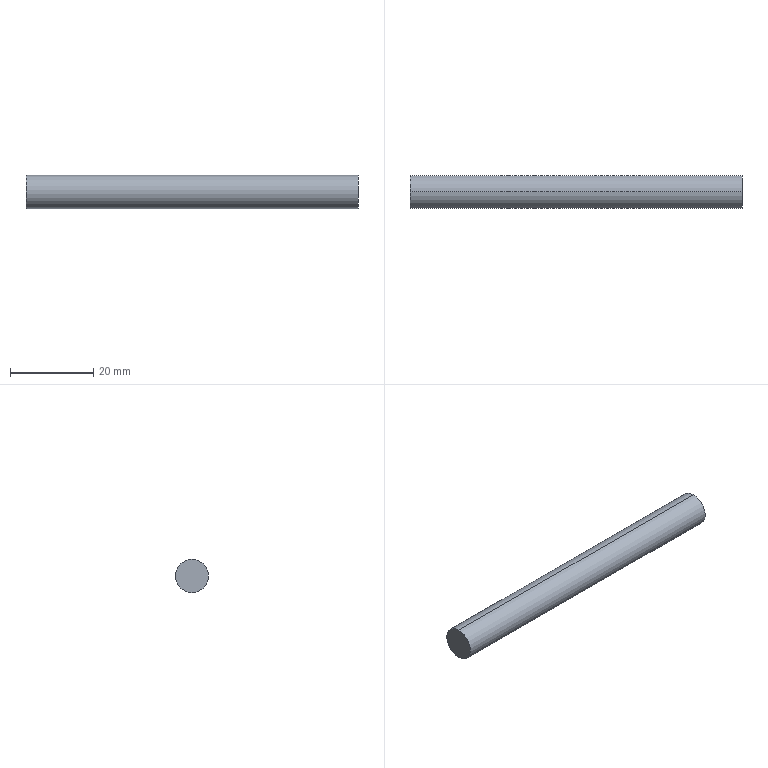Part | SolidWorks | features 3DProfileFeature 1, HoleWzd 1, Revolution 1 | 1 solid | 9 faces | box 79.975 x 8 x 8 mm | volume 3311 mm3 | cylinder 4 | cone 4 | plane 1 | commonest cylinder face diameters 6.8 x2 8 x2
STEP:
#1=CARTESIAN_POINT('',(61.25,0.,3.4));
#2=VERTEX_POINT('',#1);
#3=CARTESIAN_POINT('',(61.25,0.,-3.4));
#4=VERTEX_POINT('',#3);
#5=CARTESIAN_POINT('',(61.25,0.,0.));
#6=DIRECTION('',(1.,0.,0.));
#7=DIRECTION('',(0.,0.,-1.));
#8=AXIS2_PLACEMENT_3D('',#5,#6,#7);
#9=CIRCLE('',#8,3.4);
#10=EDGE_CURVE('',#2,#4,#9,.T.);
#11=ORIENTED_EDGE('',*,*,#10,.F.);
#12=CARTESIAN_POINT('',(79.375,0.,3.4));
#13=VERTEX_POINT('',#12);
#14=CARTESIAN_POINT('',(80.,0.,3.4));
#15=DIRECTION('',(1.,0.,0.));
#16=VECTOR('',#15,1000.);
#17=LINE('',#14,#16);
#18=EDGE_CURVE('',#2,#13,#17,.T.);
#19=ORIENTED_EDGE('',*,*,#18,.T.);
#20=CARTESIAN_POINT('',(79.375,0.,-3.4));
#21=VERTEX_POINT('',#20);
#22=CARTESIAN_POINT('',(79.375,0.,0.));
#23=DIRECTION('',(1.,0.,0.));
#24=DIRECTION('',(0.,0.,-1.));
#25=AXIS2_PLACEMENT_3D('',#22,#23,#24);
#26=CIRCLE('',#25,3.4);
#27=EDGE_CURVE('',#13,#21,#26,.T.);
#28=ORIENTED_EDGE('',*,*,#27,.T.);
#29=CARTESIAN_POINT('',(80.,0.,-3.4));
#30=DIRECTION('',(1.,0.,0.));
#31=VECTOR('',#30,1000.);
#32=LINE('',#29,#31);
#33=EDGE_CURVE('',#4,#21,#32,.T.);
#34=ORIENTED_EDGE('',*,*,#33,.F.);
#35=EDGE_LOOP('',(#11,#19,#28,#34));
#36=FACE_OUTER_BOUND('',#35,.T.);
#37=CARTESIAN_POINT('',(80.,0.,0.));
#38=DIRECTION('',(1.,0.,0.));
#39=DIRECTION('',(0.,0.,-1.));
#40=AXIS2_PLACEMENT_3D('',#37,#38,#39);
#41=CYLINDRICAL_SURFACE('',#40,3.4);
#42=ADVANCED_FACE('',(#36),#41,.F.);
#43=CARTESIAN_POINT('',(59.207,0.,0.));
#44=VERTEX_POINT('',#43);
#45=CARTESIAN_POINT('',(61.25,0.,-3.4));
#46=DIRECTION('',(0.515,0.,-0.8572));
#47=VECTOR('',#46,1000.);
#48=LINE('',#45,#47);
#49=EDGE_CURVE('',#44,#4,#48,.T.);
#50=ORIENTED_EDGE('',*,*,#49,.F.);
#51=CARTESIAN_POINT('',(61.25,0.,3.4));
#52=DIRECTION('',(0.515,0.,0.8572));
#53=VECTOR('',#52,1000.);
#54=LINE('',#51,#53);
#55=EDGE_CURVE('',#44,#2,#54,.T.);
#56=ORIENTED_EDGE('',*,*,#55,.T.);
#57=ORIENTED_EDGE('',*,*,#10,.T.);
#58=EDGE_LOOP('',(#50,#56,#57));
#59=FACE_OUTER_BOUND('',#58,.T.);
#60=CARTESIAN_POINT('',(61.25,0.,0.));
#61=DIRECTION('',(1.,0.,0.));
#62=DIRECTION('',(0.,0.,-1.));
#63=AXIS2_PLACEMENT_3D('',#60,#61,#62);
#64=CONICAL_SURFACE('',#63,3.4,1.03);
#65=ADVANCED_FACE('',(#59),#64,.F.);
#66=ORIENTED_EDGE('',*,*,#27,.F.);
#67=CARTESIAN_POINT('',(79.975,0.,4.));
#68=VERTEX_POINT('',#67);
#69=CARTESIAN_POINT('',(80.,0.,4.025));
#70=DIRECTION('',(0.7071,0.,0.7071));
#71=VECTOR('',#70,1000.);
#72=LINE('',#69,#71);
#73=EDGE_CURVE('',#13,#68,#72,.T.);
#74=ORIENTED_EDGE('',*,*,#73,.T.);
#75=CARTESIAN_POINT('',(79.975,0.,-4.));
#76=VERTEX_POINT('',#75);
#77=CARTESIAN_POINT('',(79.975,0.,0.));
#78=DIRECTION('',(-1.,0.,0.));
#79=DIRECTION('',(0.,0.,-1.));
#80=AXIS2_PLACEMENT_3D('',#77,#78,#79);
#81=CIRCLE('',#80,4.);
#82=EDGE_CURVE('',#76,#68,#81,.T.);
#83=ORIENTED_EDGE('',*,*,#82,.F.);
#84=CARTESIAN_POINT('',(80.,0.,-4.025));
#85=DIRECTION('',(0.7071,0.,-0.7071));
#86=VECTOR('',#85,1000.);
#87=LINE('',#84,#86);
#88=EDGE_CURVE('',#21,#76,#87,.T.);
#89=ORIENTED_EDGE('',*,*,#88,.F.);
#90=EDGE_LOOP('',(#66,#74,#83,#89));
#91=FACE_OUTER_BOUND('',#90,.T.);
#92=CARTESIAN_POINT('',(80.,0.,0.));
#93=DIRECTION('',(1.,0.,0.));
#94=DIRECTION('',(0.,0.,-1.));
#95=AXIS2_PLACEMENT_3D('',#92,#93,#94);
#96=CONICAL_SURFACE('',#95,4.025,0.7854);
#97=ADVANCED_FACE('',(#91),#96,.F.);
#98=CARTESIAN_POINT('',(79.975,0.,0.));
#99=DIRECTION('',(-1.,0.,0.));
#100=DIRECTION('',(0.,0.,-1.));
#101=AXIS2_PLACEMENT_3D('',#98,#99,#100);
#102=CIRCLE('',#101,4.);
#103=EDGE_CURVE('',#68,#76,#102,.T.);
#104=ORIENTED_EDGE('',*,*,#103,.T.);
#105=CARTESIAN_POINT('',(0.,0.,-4.));
#106=VERTEX_POINT('',#105);
#107=CARTESIAN_POINT('',(0.,0.,-4.));
#108=DIRECTION('',(-1.,0.,0.));
#109=VECTOR('',#108,1000.);
#110=LINE('',#107,#109);
#111=EDGE_CURVE('',#76,#106,#110,.T.);
#112=ORIENTED_EDGE('',*,*,#111,.T.);
#113=CARTESIAN_POINT('',(0.,0.,4.));
#114=VERTEX_POINT('',#113);
#115=CARTESIAN_POINT('',(0.,0.,0.));
#116=DIRECTION('',(-1.,0.,0.));
#117=DIRECTION('',(0.,0.,1.));
#118=AXIS2_PLACEMENT_3D('',#115,#116,#117);
#119=CIRCLE('',#118,4.);
#120=EDGE_CURVE('',#114,#106,#119,.T.);
#121=ORIENTED_EDGE('',*,*,#120,.F.);
#122=CARTESIAN_POINT('',(0.,0.,4.));
#123=DIRECTION('',(-1.,0.,0.));
#124=VECTOR('',#123,1000.);
#125=LINE('',#122,#124);
#126=EDGE_CURVE('',#68,#114,#125,.T.);
#127=ORIENTED_EDGE('',*,*,#126,.F.);
#128=EDGE_LOOP('',(#104,#112,#121,#127));
#129=FACE_OUTER_BOUND('',#128,.T.);
#130=CARTESIAN_POINT('',(0.,0.,0.));
#131=DIRECTION('',(-1.,0.,0.));
#132=DIRECTION('',(0.,0.,1.));
#133=AXIS2_PLACEMENT_3D('',#130,#131,#132);
#134=CYLINDRICAL_SURFACE('',#133,4.);
#135=ADVANCED_FACE('',(#129),#134,.T.);
#136=ORIENTED_EDGE('',*,*,#120,.T.);
#137=CARTESIAN_POINT('',(0.,0.,0.));
#138=DIRECTION('',(-1.,0.,0.));
#139=DIRECTION('',(0.,0.,1.));
#140=AXIS2_PLACEMENT_3D('',#137,#138,#139);
#141=CIRCLE('',#140,4.);
#142=EDGE_CURVE('',#106,#114,#141,.T.);
#143=ORIENTED_EDGE('',*,*,#142,.T.);
#144=EDGE_LOOP('',(#136,#143));
#145=FACE_OUTER_BOUND('',#144,.T.);
#146=CARTESIAN_POINT('',(0.,0.,0.));
#147=DIRECTION('',(1.,0.,0.));
#148=DIRECTION('',(0.,0.,-1.));
#149=AXIS2_PLACEMENT_3D('',#146,#147,#148);
#150=PLANE('',#149);
#151=ADVANCED_FACE('',(#145),#150,.F.);
#152=ORIENTED_EDGE('',*,*,#111,.F.);
#153=ORIENTED_EDGE('',*,*,#82,.T.);
#154=ORIENTED_EDGE('',*,*,#126,.T.);
#155=ORIENTED_EDGE('',*,*,#142,.F.);
#156=EDGE_LOOP('',(#152,#153,#154,#155));
#157=FACE_OUTER_BOUND('',#156,.T.);
#158=CARTESIAN_POINT('',(0.,0.,0.));
#159=DIRECTION('',(-1.,0.,0.));
#160=DIRECTION('',(0.,0.,1.));
#161=AXIS2_PLACEMENT_3D('',#158,#159,#160);
#162=CYLINDRICAL_SURFACE('',#161,4.);
#163=ADVANCED_FACE('',(#157),#162,.T.);
#164=ORIENTED_EDGE('',*,*,#73,.F.);
#165=CARTESIAN_POINT('',(79.375,0.,0.));
#166=DIRECTION('',(1.,0.,0.));
#167=DIRECTION('',(0.,0.,-1.));
#168=AXIS2_PLACEMENT_3D('',#165,#166,#167);
#169=CIRCLE('',#168,3.4);
#170=EDGE_CURVE('',#21,#13,#169,.T.);
#171=ORIENTED_EDGE('',*,*,#170,.F.);
#172=ORIENTED_EDGE('',*,*,#88,.T.);
#173=ORIENTED_EDGE('',*,*,#103,.F.);
#174=EDGE_LOOP('',(#164,#171,#172,#173));
#175=FACE_OUTER_BOUND('',#174,.T.);
#176=CARTESIAN_POINT('',(80.,0.,0.));
#177=DIRECTION('',(1.,0.,0.));
#178=DIRECTION('',(0.,0.,-1.));
#179=AXIS2_PLACEMENT_3D('',#176,#177,#178);
#180=CONICAL_SURFACE('',#179,4.025,0.7854);
#181=ADVANCED_FACE('',(#175),#180,.F.);
#182=ORIENTED_EDGE('',*,*,#55,.F.);
#183=ORIENTED_EDGE('',*,*,#49,.T.);
#184=CARTESIAN_POINT('',(61.25,0.,0.));
#185=DIRECTION('',(1.,0.,0.));
#186=DIRECTION('',(0.,0.,-1.));
#187=AXIS2_PLACEMENT_3D('',#184,#185,#186);
#188=CIRCLE('',#187,3.4);
#189=EDGE_CURVE('',#4,#2,#188,.T.);
#190=ORIENTED_EDGE('',*,*,#189,.T.);
#191=EDGE_LOOP('',(#182,#183,#190));
#192=FACE_OUTER_BOUND('',#191,.T.);
#193=CARTESIAN_POINT('',(61.25,0.,0.));
#194=DIRECTION('',(1.,0.,0.));
#195=DIRECTION('',(0.,0.,-1.));
#196=AXIS2_PLACEMENT_3D('',#193,#194,#195);
#197=CONICAL_SURFACE('',#196,3.4,1.03);
#198=ADVANCED_FACE('',(#192),#197,.F.);
#199=ORIENTED_EDGE('',*,*,#18,.F.);
#200=ORIENTED_EDGE('',*,*,#189,.F.);
#201=ORIENTED_EDGE('',*,*,#33,.T.);
#202=ORIENTED_EDGE('',*,*,#170,.T.);
#203=EDGE_LOOP('',(#199,#200,#201,#202));
#204=FACE_OUTER_BOUND('',#203,.T.);
#205=CARTESIAN_POINT('',(80.,0.,0.));
#206=DIRECTION('',(1.,0.,0.));
#207=DIRECTION('',(0.,0.,-1.));
#208=AXIS2_PLACEMENT_3D('',#205,#206,#207);
#209=CYLINDRICAL_SURFACE('',#208,3.4);
#210=ADVANCED_FACE('',(#204),#209,.F.);
#211=CLOSED_SHELL('',(#42,#65,#97,#135,#151,#163,#181,#198,#210));
#212=MANIFOLD_SOLID_BREP('',#211);
#213=CARTESIAN_POINT('',(0.,0.,0.));
#214=DIRECTION('',(0.,0.,1.));
#215=DIRECTION('',(1.,0.,0.));
#216=AXIS2_PLACEMENT_3D('',#213,#214,#215);
#217=(LENGTH_UNIT()NAMED_UNIT(*)SI_UNIT(.MILLI.,.METRE.));
#218=UNCERTAINTY_MEASURE_WITH_UNIT(LENGTH_MEASURE(0.00001),#217,'','');
#219=(NAMED_UNIT(*)PLANE_ANGLE_UNIT()SI_UNIT($,.RADIAN.));
#220=(NAMED_UNIT(*)SI_UNIT($,.STERADIAN.)SOLID_ANGLE_UNIT());
#221=(GEOMETRIC_REPRESENTATION_CONTEXT(3)GLOBAL_UNCERTAINTY_ASSIGNED_CONTEXT((#218))GLOBAL_UNIT_ASSIGNED_CONTEXT((#217,#219,#220))REPRESENTATION_CONTEXT('',''));
#222=ADVANCED_BREP_SHAPE_REPRESENTATION('',(#212,#216),#221);